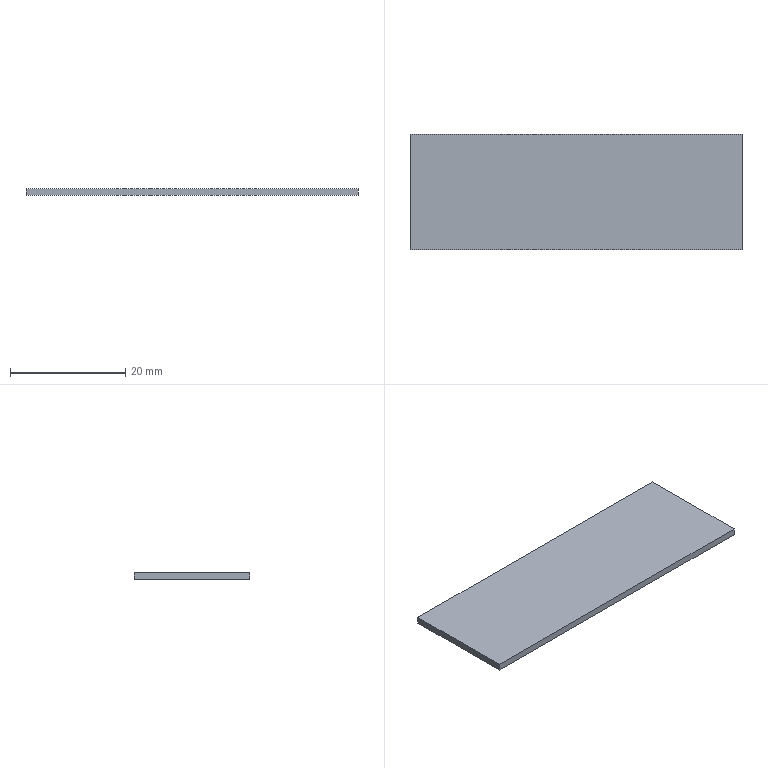Part | SolidWorks | features BaseBody 1 | 1 solid | 6 faces | box 57.6 x 20 x 1.2 mm | volume 1382 mm3 | plane 6
STEP:
#1=CARTESIAN_POINT('',(-28.8,10.,0.));
#2=VERTEX_POINT('',#1);
#3=CARTESIAN_POINT('',(-28.8,-10.,0.));
#4=VERTEX_POINT('',#3);
#5=CARTESIAN_POINT('',(-28.8,10.,0.));
#6=DIRECTION('',(0.,-1.,0.));
#7=VECTOR('',#6,1000.);
#8=LINE('',#5,#7);
#9=EDGE_CURVE('',#2,#4,#8,.T.);
#10=ORIENTED_EDGE('',*,*,#9,.T.);
#11=CARTESIAN_POINT('',(28.8,-10.,0.));
#12=VERTEX_POINT('',#11);
#13=CARTESIAN_POINT('',(28.8,-10.,0.));
#14=DIRECTION('',(1.,0.,0.));
#15=VECTOR('',#14,1000.);
#16=LINE('',#13,#15);
#17=EDGE_CURVE('',#4,#12,#16,.T.);
#18=ORIENTED_EDGE('',*,*,#17,.T.);
#19=CARTESIAN_POINT('',(28.8,10.,0.));
#20=VERTEX_POINT('',#19);
#21=CARTESIAN_POINT('',(28.8,10.,0.));
#22=DIRECTION('',(0.,1.,0.));
#23=VECTOR('',#22,1000.);
#24=LINE('',#21,#23);
#25=EDGE_CURVE('',#12,#20,#24,.T.);
#26=ORIENTED_EDGE('',*,*,#25,.T.);
#27=CARTESIAN_POINT('',(28.8,10.,0.));
#28=DIRECTION('',(-1.,0.,0.));
#29=VECTOR('',#28,1000.);
#30=LINE('',#27,#29);
#31=EDGE_CURVE('',#20,#2,#30,.T.);
#32=ORIENTED_EDGE('',*,*,#31,.T.);
#33=EDGE_LOOP('',(#10,#18,#26,#32));
#34=FACE_OUTER_BOUND('',#33,.T.);
#35=CARTESIAN_POINT('',(0.,0.,0.));
#36=DIRECTION('',(0.,0.,-1.));
#37=DIRECTION('',(0.,-1.,0.));
#38=AXIS2_PLACEMENT_3D('',#35,#36,#37);
#39=PLANE('',#38);
#40=ADVANCED_FACE('',(#34),#39,.F.);
#41=CARTESIAN_POINT('',(-28.8,10.,-1.2));
#42=VERTEX_POINT('',#41);
#43=CARTESIAN_POINT('',(-28.8,-10.,-1.2));
#44=VERTEX_POINT('',#43);
#45=CARTESIAN_POINT('',(-28.8,10.,-1.2));
#46=DIRECTION('',(0.,-1.,0.));
#47=VECTOR('',#46,1000.);
#48=LINE('',#45,#47);
#49=EDGE_CURVE('',#42,#44,#48,.T.);
#50=ORIENTED_EDGE('',*,*,#49,.F.);
#51=CARTESIAN_POINT('',(28.8,10.,-1.2));
#52=VERTEX_POINT('',#51);
#53=CARTESIAN_POINT('',(28.8,10.,-1.2));
#54=DIRECTION('',(-1.,0.,0.));
#55=VECTOR('',#54,1000.);
#56=LINE('',#53,#55);
#57=EDGE_CURVE('',#52,#42,#56,.T.);
#58=ORIENTED_EDGE('',*,*,#57,.F.);
#59=CARTESIAN_POINT('',(28.8,-10.,-1.2));
#60=VERTEX_POINT('',#59);
#61=CARTESIAN_POINT('',(28.8,10.,-1.2));
#62=DIRECTION('',(0.,1.,0.));
#63=VECTOR('',#62,1000.);
#64=LINE('',#61,#63);
#65=EDGE_CURVE('',#60,#52,#64,.T.);
#66=ORIENTED_EDGE('',*,*,#65,.F.);
#67=CARTESIAN_POINT('',(28.8,-10.,-1.2));
#68=DIRECTION('',(1.,0.,0.));
#69=VECTOR('',#68,1000.);
#70=LINE('',#67,#69);
#71=EDGE_CURVE('',#44,#60,#70,.T.);
#72=ORIENTED_EDGE('',*,*,#71,.F.);
#73=EDGE_LOOP('',(#50,#58,#66,#72));
#74=FACE_OUTER_BOUND('',#73,.T.);
#75=CARTESIAN_POINT('',(0.,0.,-1.2));
#76=DIRECTION('',(0.,0.,-1.));
#77=DIRECTION('',(0.,-1.,0.));
#78=AXIS2_PLACEMENT_3D('',#75,#76,#77);
#79=PLANE('',#78);
#80=ADVANCED_FACE('',(#74),#79,.T.);
#81=ORIENTED_EDGE('',*,*,#17,.F.);
#82=CARTESIAN_POINT('',(-28.8,-10.,-1.2));
#83=DIRECTION('',(0.,0.,1.));
#84=VECTOR('',#83,1000.);
#85=LINE('',#82,#84);
#86=EDGE_CURVE('',#44,#4,#85,.T.);
#87=ORIENTED_EDGE('',*,*,#86,.F.);
#88=ORIENTED_EDGE('',*,*,#71,.T.);
#89=CARTESIAN_POINT('',(28.8,-10.,-1.2));
#90=DIRECTION('',(0.,0.,1.));
#91=VECTOR('',#90,1000.);
#92=LINE('',#89,#91);
#93=EDGE_CURVE('',#60,#12,#92,.T.);
#94=ORIENTED_EDGE('',*,*,#93,.T.);
#95=EDGE_LOOP('',(#81,#87,#88,#94));
#96=FACE_OUTER_BOUND('',#95,.T.);
#97=CARTESIAN_POINT('',(28.8,-10.,-1.2));
#98=DIRECTION('',(0.,-1.,0.));
#99=DIRECTION('',(0.,0.,-1.));
#100=AXIS2_PLACEMENT_3D('',#97,#98,#99);
#101=PLANE('',#100);
#102=ADVANCED_FACE('',(#96),#101,.T.);
#103=ORIENTED_EDGE('',*,*,#25,.F.);
#104=ORIENTED_EDGE('',*,*,#93,.F.);
#105=ORIENTED_EDGE('',*,*,#65,.T.);
#106=CARTESIAN_POINT('',(28.8,10.,-1.2));
#107=DIRECTION('',(0.,0.,1.));
#108=VECTOR('',#107,1000.);
#109=LINE('',#106,#108);
#110=EDGE_CURVE('',#52,#20,#109,.T.);
#111=ORIENTED_EDGE('',*,*,#110,.T.);
#112=EDGE_LOOP('',(#103,#104,#105,#111));
#113=FACE_OUTER_BOUND('',#112,.T.);
#114=CARTESIAN_POINT('',(28.8,10.,-1.2));
#115=DIRECTION('',(1.,0.,0.));
#116=DIRECTION('',(0.,1.,0.));
#117=AXIS2_PLACEMENT_3D('',#114,#115,#116);
#118=PLANE('',#117);
#119=ADVANCED_FACE('',(#113),#118,.T.);
#120=ORIENTED_EDGE('',*,*,#31,.F.);
#121=ORIENTED_EDGE('',*,*,#110,.F.);
#122=ORIENTED_EDGE('',*,*,#57,.T.);
#123=CARTESIAN_POINT('',(-28.8,10.,-1.2));
#124=DIRECTION('',(0.,0.,1.));
#125=VECTOR('',#124,1000.);
#126=LINE('',#123,#125);
#127=EDGE_CURVE('',#42,#2,#126,.T.);
#128=ORIENTED_EDGE('',*,*,#127,.T.);
#129=EDGE_LOOP('',(#120,#121,#122,#128));
#130=FACE_OUTER_BOUND('',#129,.T.);
#131=CARTESIAN_POINT('',(28.8,10.,-1.2));
#132=DIRECTION('',(0.,1.,0.));
#133=DIRECTION('',(1.,0.,0.));
#134=AXIS2_PLACEMENT_3D('',#131,#132,#133);
#135=PLANE('',#134);
#136=ADVANCED_FACE('',(#130),#135,.T.);
#137=ORIENTED_EDGE('',*,*,#9,.F.);
#138=ORIENTED_EDGE('',*,*,#127,.F.);
#139=ORIENTED_EDGE('',*,*,#49,.T.);
#140=ORIENTED_EDGE('',*,*,#86,.T.);
#141=EDGE_LOOP('',(#137,#138,#139,#140));
#142=FACE_OUTER_BOUND('',#141,.T.);
#143=CARTESIAN_POINT('',(-28.8,10.,-1.2));
#144=DIRECTION('',(-1.,0.,0.));
#145=DIRECTION('',(0.,0.,1.));
#146=AXIS2_PLACEMENT_3D('',#143,#144,#145);
#147=PLANE('',#146);
#148=ADVANCED_FACE('',(#142),#147,.T.);
#149=CLOSED_SHELL('',(#40,#80,#102,#119,#136,#148));
#150=MANIFOLD_SOLID_BREP('',#149);
#151=CARTESIAN_POINT('',(0.,0.,0.));
#152=DIRECTION('',(0.,0.,1.));
#153=DIRECTION('',(1.,0.,0.));
#154=AXIS2_PLACEMENT_3D('',#151,#152,#153);
#155=(LENGTH_UNIT()NAMED_UNIT(*)SI_UNIT(.MILLI.,.METRE.));
#156=UNCERTAINTY_MEASURE_WITH_UNIT(LENGTH_MEASURE(0.00001),#155,'','');
#157=(NAMED_UNIT(*)PLANE_ANGLE_UNIT()SI_UNIT($,.RADIAN.));
#158=(NAMED_UNIT(*)SI_UNIT($,.STERADIAN.)SOLID_ANGLE_UNIT());
#159=(GEOMETRIC_REPRESENTATION_CONTEXT(3)GLOBAL_UNCERTAINTY_ASSIGNED_CONTEXT((#156))GLOBAL_UNIT_ASSIGNED_CONTEXT((#155,#157,#158))REPRESENTATION_CONTEXT('',''));
#160=ADVANCED_BREP_SHAPE_REPRESENTATION('',(#150,#154),#159);